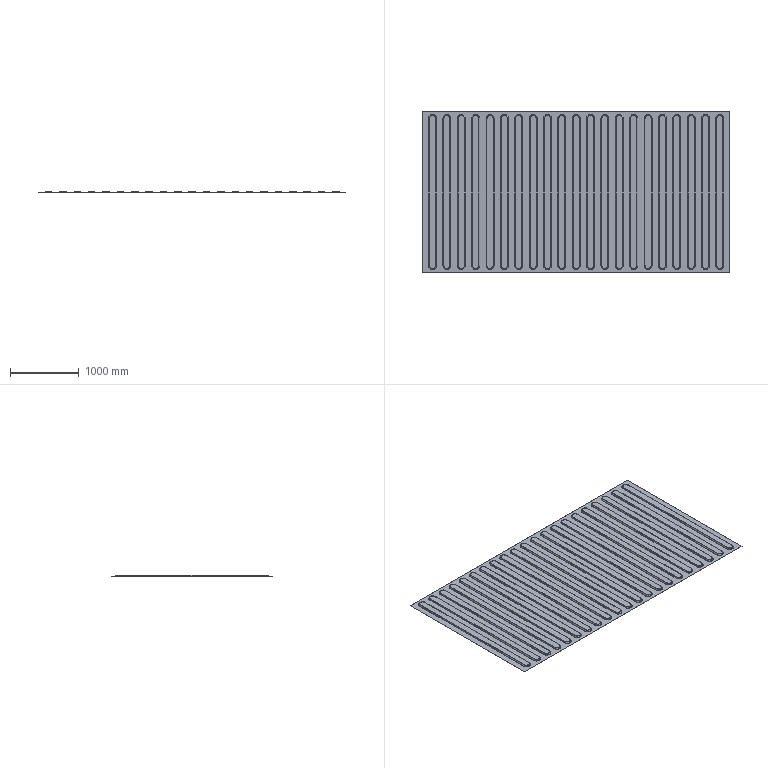Part | STEP file | 750038167 | 1 solid | 558 faces | box 4475 x 2356 x 19.9 mm | volume 17264106 mm3 | spline 168 | cylinder 168 | plane 132 | cone 90 | commonest cylinder face diameters 4 x84 7 x84